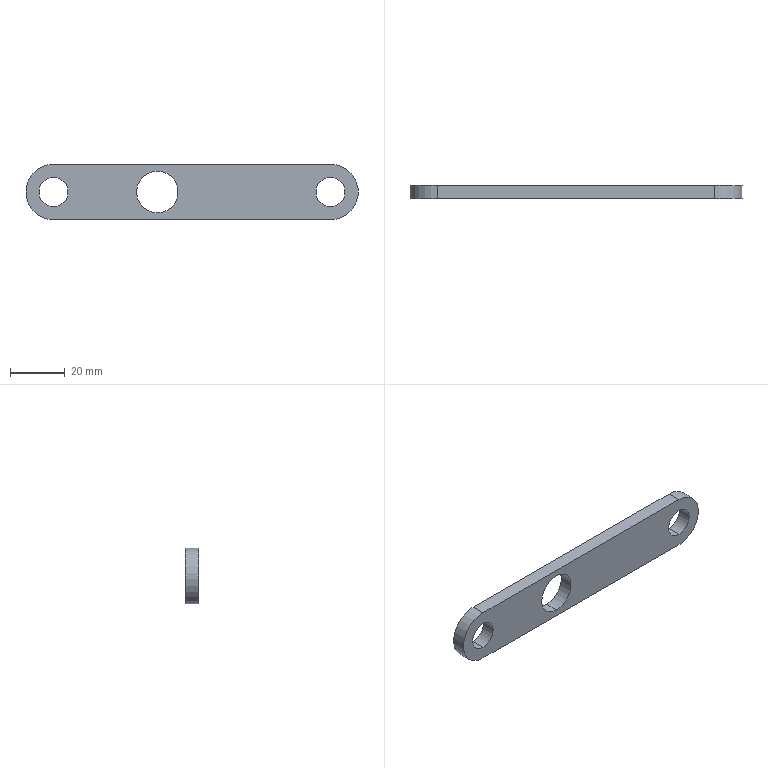Part | SolidWorks | features Extrusion 1, Scale 1 | 1 solid | 12 faces | box 121.92 x 5.08 x 20.32 mm | volume 10300 mm3 | cylinder 8 | plane 4 | commonest cylinder face diameters 10.668 x4 15.24 x2 20.32 x2
STEP:
#1=CARTESIAN_POINT('',(-12.7,5.08,-7.62));
#2=VERTEX_POINT('',#1);
#3=CARTESIAN_POINT('',(-12.7,5.08,7.62));
#4=VERTEX_POINT('',#3);
#5=CARTESIAN_POINT('',(-12.7,5.08,0.));
#6=DIRECTION('',(0.,1.,0.));
#7=DIRECTION('',(0.,0.,1.));
#8=AXIS2_PLACEMENT_3D('',#5,#6,#7);
#9=CIRCLE('',#8,7.62);
#10=EDGE_CURVE('',#2,#4,#9,.T.);
#11=ORIENTED_EDGE('',*,*,#10,.T.);
#12=CARTESIAN_POINT('',(-12.7,0.,7.62));
#13=VERTEX_POINT('',#12);
#14=CARTESIAN_POINT('',(-12.7,5.08,7.62));
#15=DIRECTION('',(0.,-1.,0.));
#16=VECTOR('',#15,1000.);
#17=LINE('',#14,#16);
#18=EDGE_CURVE('',#4,#13,#17,.T.);
#19=ORIENTED_EDGE('',*,*,#18,.T.);
#20=CARTESIAN_POINT('',(-12.7,0.,-7.62));
#21=VERTEX_POINT('',#20);
#22=CARTESIAN_POINT('',(-12.7,0.,0.));
#23=DIRECTION('',(0.,1.,0.));
#24=DIRECTION('',(0.,0.,1.));
#25=AXIS2_PLACEMENT_3D('',#22,#23,#24);
#26=CIRCLE('',#25,7.62);
#27=EDGE_CURVE('',#21,#13,#26,.T.);
#28=ORIENTED_EDGE('',*,*,#27,.F.);
#29=CARTESIAN_POINT('',(-12.7,5.08,-7.62));
#30=DIRECTION('',(0.,-1.,0.));
#31=VECTOR('',#30,1000.);
#32=LINE('',#29,#31);
#33=EDGE_CURVE('',#2,#21,#32,.T.);
#34=ORIENTED_EDGE('',*,*,#33,.F.);
#35=EDGE_LOOP('',(#11,#19,#28,#34));
#36=FACE_OUTER_BOUND('',#35,.T.);
#37=CARTESIAN_POINT('',(-12.7,5.08,0.));
#38=DIRECTION('',(0.,-1.,0.));
#39=DIRECTION('',(0.,0.,-1.));
#40=AXIS2_PLACEMENT_3D('',#37,#38,#39);
#41=CYLINDRICAL_SURFACE('',#40,7.62);
#42=ADVANCED_FACE('',(#36),#41,.F.);
#43=CARTESIAN_POINT('',(50.8,5.08,-5.334));
#44=VERTEX_POINT('',#43);
#45=CARTESIAN_POINT('',(50.8,5.08,5.334));
#46=VERTEX_POINT('',#45);
#47=CARTESIAN_POINT('',(50.8,5.08,0.));
#48=DIRECTION('',(0.,1.,0.));
#49=DIRECTION('',(0.,0.,1.));
#50=AXIS2_PLACEMENT_3D('',#47,#48,#49);
#51=CIRCLE('',#50,5.334);
#52=EDGE_CURVE('',#44,#46,#51,.T.);
#53=ORIENTED_EDGE('',*,*,#52,.T.);
#54=CARTESIAN_POINT('',(50.8,0.,5.334));
#55=VERTEX_POINT('',#54);
#56=CARTESIAN_POINT('',(50.8,5.08,5.334));
#57=DIRECTION('',(0.,-1.,0.));
#58=VECTOR('',#57,1000.);
#59=LINE('',#56,#58);
#60=EDGE_CURVE('',#46,#55,#59,.T.);
#61=ORIENTED_EDGE('',*,*,#60,.T.);
#62=CARTESIAN_POINT('',(50.8,0.,-5.334));
#63=VERTEX_POINT('',#62);
#64=CARTESIAN_POINT('',(50.8,0.,0.));
#65=DIRECTION('',(0.,1.,0.));
#66=DIRECTION('',(0.,0.,1.));
#67=AXIS2_PLACEMENT_3D('',#64,#65,#66);
#68=CIRCLE('',#67,5.334);
#69=EDGE_CURVE('',#63,#55,#68,.T.);
#70=ORIENTED_EDGE('',*,*,#69,.F.);
#71=CARTESIAN_POINT('',(50.8,5.08,-5.334));
#72=DIRECTION('',(0.,-1.,0.));
#73=VECTOR('',#72,1000.);
#74=LINE('',#71,#73);
#75=EDGE_CURVE('',#44,#63,#74,.T.);
#76=ORIENTED_EDGE('',*,*,#75,.F.);
#77=EDGE_LOOP('',(#53,#61,#70,#76));
#78=FACE_OUTER_BOUND('',#77,.T.);
#79=CARTESIAN_POINT('',(50.8,5.08,0.));
#80=DIRECTION('',(0.,-1.,0.));
#81=DIRECTION('',(0.,0.,-1.));
#82=AXIS2_PLACEMENT_3D('',#79,#80,#81);
#83=CYLINDRICAL_SURFACE('',#82,5.334);
#84=ADVANCED_FACE('',(#78),#83,.F.);
#85=CARTESIAN_POINT('',(-50.8,5.08,-5.334));
#86=VERTEX_POINT('',#85);
#87=CARTESIAN_POINT('',(-50.8,5.08,5.334));
#88=VERTEX_POINT('',#87);
#89=CARTESIAN_POINT('',(-50.8,5.08,0.));
#90=DIRECTION('',(0.,1.,0.));
#91=DIRECTION('',(0.,0.,1.));
#92=AXIS2_PLACEMENT_3D('',#89,#90,#91);
#93=CIRCLE('',#92,5.334);
#94=EDGE_CURVE('',#86,#88,#93,.T.);
#95=ORIENTED_EDGE('',*,*,#94,.T.);
#96=CARTESIAN_POINT('',(-50.8,0.,5.334));
#97=VERTEX_POINT('',#96);
#98=CARTESIAN_POINT('',(-50.8,5.08,5.334));
#99=DIRECTION('',(0.,-1.,0.));
#100=VECTOR('',#99,1000.);
#101=LINE('',#98,#100);
#102=EDGE_CURVE('',#88,#97,#101,.T.);
#103=ORIENTED_EDGE('',*,*,#102,.T.);
#104=CARTESIAN_POINT('',(-50.8,0.,-5.334));
#105=VERTEX_POINT('',#104);
#106=CARTESIAN_POINT('',(-50.8,0.,0.));
#107=DIRECTION('',(0.,1.,0.));
#108=DIRECTION('',(0.,0.,1.));
#109=AXIS2_PLACEMENT_3D('',#106,#107,#108);
#110=CIRCLE('',#109,5.334);
#111=EDGE_CURVE('',#105,#97,#110,.T.);
#112=ORIENTED_EDGE('',*,*,#111,.F.);
#113=CARTESIAN_POINT('',(-50.8,5.08,-5.334));
#114=DIRECTION('',(0.,-1.,0.));
#115=VECTOR('',#114,1000.);
#116=LINE('',#113,#115);
#117=EDGE_CURVE('',#86,#105,#116,.T.);
#118=ORIENTED_EDGE('',*,*,#117,.F.);
#119=EDGE_LOOP('',(#95,#103,#112,#118));
#120=FACE_OUTER_BOUND('',#119,.T.);
#121=CARTESIAN_POINT('',(-50.8,5.08,0.));
#122=DIRECTION('',(0.,-1.,0.));
#123=DIRECTION('',(0.,0.,-1.));
#124=AXIS2_PLACEMENT_3D('',#121,#122,#123);
#125=CYLINDRICAL_SURFACE('',#124,5.334);
#126=ADVANCED_FACE('',(#120),#125,.F.);
#127=ORIENTED_EDGE('',*,*,#52,.F.);
#128=CARTESIAN_POINT('',(50.8,5.08,0.));
#129=DIRECTION('',(0.,1.,0.));
#130=DIRECTION('',(0.,0.,1.));
#131=AXIS2_PLACEMENT_3D('',#128,#129,#130);
#132=CIRCLE('',#131,5.334);
#133=EDGE_CURVE('',#46,#44,#132,.T.);
#134=ORIENTED_EDGE('',*,*,#133,.F.);
#135=EDGE_LOOP('',(#127,#134));
#136=FACE_BOUND('',#135,.T.);
#137=CARTESIAN_POINT('',(-50.8,5.08,-10.16));
#138=VERTEX_POINT('',#137);
#139=CARTESIAN_POINT('',(-50.8,5.08,10.16));
#140=VERTEX_POINT('',#139);
#141=CARTESIAN_POINT('',(-50.8,5.08,0.));
#142=DIRECTION('',(0.,1.,0.));
#143=DIRECTION('',(0.,0.,1.));
#144=AXIS2_PLACEMENT_3D('',#141,#142,#143);
#145=CIRCLE('',#144,10.16);
#146=EDGE_CURVE('',#138,#140,#145,.T.);
#147=ORIENTED_EDGE('',*,*,#146,.T.);
#148=CARTESIAN_POINT('',(50.8,5.08,10.16));
#149=VERTEX_POINT('',#148);
#150=CARTESIAN_POINT('',(-50.8,5.08,10.16));
#151=DIRECTION('',(1.,0.,0.));
#152=VECTOR('',#151,1000.);
#153=LINE('',#150,#152);
#154=EDGE_CURVE('',#140,#149,#153,.T.);
#155=ORIENTED_EDGE('',*,*,#154,.T.);
#156=CARTESIAN_POINT('',(50.8,5.08,-10.16));
#157=VERTEX_POINT('',#156);
#158=CARTESIAN_POINT('',(50.8,5.08,0.));
#159=DIRECTION('',(0.,1.,0.));
#160=DIRECTION('',(0.,0.,1.));
#161=AXIS2_PLACEMENT_3D('',#158,#159,#160);
#162=CIRCLE('',#161,10.16);
#163=EDGE_CURVE('',#149,#157,#162,.T.);
#164=ORIENTED_EDGE('',*,*,#163,.T.);
#165=CARTESIAN_POINT('',(-50.8,5.08,-10.16));
#166=DIRECTION('',(-1.,0.,0.));
#167=VECTOR('',#166,1000.);
#168=LINE('',#165,#167);
#169=EDGE_CURVE('',#157,#138,#168,.T.);
#170=ORIENTED_EDGE('',*,*,#169,.T.);
#171=EDGE_LOOP('',(#147,#155,#164,#170));
#172=FACE_OUTER_BOUND('',#171,.T.);
#173=ORIENTED_EDGE('',*,*,#94,.F.);
#174=CARTESIAN_POINT('',(-50.8,5.08,0.));
#175=DIRECTION('',(0.,1.,0.));
#176=DIRECTION('',(0.,0.,1.));
#177=AXIS2_PLACEMENT_3D('',#174,#175,#176);
#178=CIRCLE('',#177,5.334);
#179=EDGE_CURVE('',#88,#86,#178,.T.);
#180=ORIENTED_EDGE('',*,*,#179,.F.);
#181=EDGE_LOOP('',(#173,#180));
#182=FACE_BOUND('',#181,.T.);
#183=ORIENTED_EDGE('',*,*,#10,.F.);
#184=CARTESIAN_POINT('',(-12.7,5.08,0.));
#185=DIRECTION('',(0.,1.,0.));
#186=DIRECTION('',(0.,0.,1.));
#187=AXIS2_PLACEMENT_3D('',#184,#185,#186);
#188=CIRCLE('',#187,7.62);
#189=EDGE_CURVE('',#4,#2,#188,.T.);
#190=ORIENTED_EDGE('',*,*,#189,.F.);
#191=EDGE_LOOP('',(#183,#190));
#192=FACE_BOUND('',#191,.T.);
#193=CARTESIAN_POINT('',(-50.8,5.08,0.));
#194=DIRECTION('',(0.,1.,0.));
#195=DIRECTION('',(0.,0.,1.));
#196=AXIS2_PLACEMENT_3D('',#193,#194,#195);
#197=PLANE('',#196);
#198=ADVANCED_FACE('',(#136,#172,#182,#192),#197,.T.);
#199=ORIENTED_EDGE('',*,*,#69,.T.);
#200=CARTESIAN_POINT('',(50.8,0.,0.));
#201=DIRECTION('',(0.,1.,0.));
#202=DIRECTION('',(0.,0.,1.));
#203=AXIS2_PLACEMENT_3D('',#200,#201,#202);
#204=CIRCLE('',#203,5.334);
#205=EDGE_CURVE('',#55,#63,#204,.T.);
#206=ORIENTED_EDGE('',*,*,#205,.T.);
#207=EDGE_LOOP('',(#199,#206));
#208=FACE_BOUND('',#207,.T.);
#209=CARTESIAN_POINT('',(-50.8,0.,-10.16));
#210=VERTEX_POINT('',#209);
#211=CARTESIAN_POINT('',(-50.8,0.,10.16));
#212=VERTEX_POINT('',#211);
#213=CARTESIAN_POINT('',(-50.8,0.,0.));
#214=DIRECTION('',(0.,1.,0.));
#215=DIRECTION('',(0.,0.,1.));
#216=AXIS2_PLACEMENT_3D('',#213,#214,#215);
#217=CIRCLE('',#216,10.16);
#218=EDGE_CURVE('',#210,#212,#217,.T.);
#219=ORIENTED_EDGE('',*,*,#218,.F.);
#220=CARTESIAN_POINT('',(50.8,0.,-10.16));
#221=VERTEX_POINT('',#220);
#222=CARTESIAN_POINT('',(-50.8,0.,-10.16));
#223=DIRECTION('',(-1.,0.,0.));
#224=VECTOR('',#223,1000.);
#225=LINE('',#222,#224);
#226=EDGE_CURVE('',#221,#210,#225,.T.);
#227=ORIENTED_EDGE('',*,*,#226,.F.);
#228=CARTESIAN_POINT('',(50.8,0.,10.16));
#229=VERTEX_POINT('',#228);
#230=CARTESIAN_POINT('',(50.8,0.,0.));
#231=DIRECTION('',(0.,1.,0.));
#232=DIRECTION('',(0.,0.,1.));
#233=AXIS2_PLACEMENT_3D('',#230,#231,#232);
#234=CIRCLE('',#233,10.16);
#235=EDGE_CURVE('',#229,#221,#234,.T.);
#236=ORIENTED_EDGE('',*,*,#235,.F.);
#237=CARTESIAN_POINT('',(-50.8,0.,10.16));
#238=DIRECTION('',(1.,0.,0.));
#239=VECTOR('',#238,1000.);
#240=LINE('',#237,#239);
#241=EDGE_CURVE('',#212,#229,#240,.T.);
#242=ORIENTED_EDGE('',*,*,#241,.F.);
#243=EDGE_LOOP('',(#219,#227,#236,#242));
#244=FACE_OUTER_BOUND('',#243,.T.);
#245=ORIENTED_EDGE('',*,*,#111,.T.);
#246=CARTESIAN_POINT('',(-50.8,0.,0.));
#247=DIRECTION('',(0.,1.,0.));
#248=DIRECTION('',(0.,0.,1.));
#249=AXIS2_PLACEMENT_3D('',#246,#247,#248);
#250=CIRCLE('',#249,5.334);
#251=EDGE_CURVE('',#97,#105,#250,.T.);
#252=ORIENTED_EDGE('',*,*,#251,.T.);
#253=EDGE_LOOP('',(#245,#252));
#254=FACE_BOUND('',#253,.T.);
#255=ORIENTED_EDGE('',*,*,#27,.T.);
#256=CARTESIAN_POINT('',(-12.7,0.,0.));
#257=DIRECTION('',(0.,1.,0.));
#258=DIRECTION('',(0.,0.,1.));
#259=AXIS2_PLACEMENT_3D('',#256,#257,#258);
#260=CIRCLE('',#259,7.62);
#261=EDGE_CURVE('',#13,#21,#260,.T.);
#262=ORIENTED_EDGE('',*,*,#261,.T.);
#263=EDGE_LOOP('',(#255,#262));
#264=FACE_BOUND('',#263,.T.);
#265=CARTESIAN_POINT('',(-50.8,0.,0.));
#266=DIRECTION('',(0.,1.,0.));
#267=DIRECTION('',(0.,0.,1.));
#268=AXIS2_PLACEMENT_3D('',#265,#266,#267);
#269=PLANE('',#268);
#270=ADVANCED_FACE('',(#208,#244,#254,#264),#269,.F.);
#271=ORIENTED_EDGE('',*,*,#218,.T.);
#272=CARTESIAN_POINT('',(-50.8,5.08,10.16));
#273=DIRECTION('',(0.,-1.,0.));
#274=VECTOR('',#273,1000.);
#275=LINE('',#272,#274);
#276=EDGE_CURVE('',#140,#212,#275,.T.);
#277=ORIENTED_EDGE('',*,*,#276,.F.);
#278=ORIENTED_EDGE('',*,*,#146,.F.);
#279=CARTESIAN_POINT('',(-50.8,5.08,-10.16));
#280=DIRECTION('',(0.,-1.,0.));
#281=VECTOR('',#280,1000.);
#282=LINE('',#279,#281);
#283=EDGE_CURVE('',#138,#210,#282,.T.);
#284=ORIENTED_EDGE('',*,*,#283,.T.);
#285=EDGE_LOOP('',(#271,#277,#278,#284));
#286=FACE_OUTER_BOUND('',#285,.T.);
#287=CARTESIAN_POINT('',(-50.8,5.08,0.));
#288=DIRECTION('',(0.,-1.,0.));
#289=DIRECTION('',(0.,0.,-1.));
#290=AXIS2_PLACEMENT_3D('',#287,#288,#289);
#291=CYLINDRICAL_SURFACE('',#290,10.16);
#292=ADVANCED_FACE('',(#286),#291,.T.);
#293=ORIENTED_EDGE('',*,*,#241,.T.);
#294=CARTESIAN_POINT('',(50.8,5.08,10.16));
#295=DIRECTION('',(0.,-1.,0.));
#296=VECTOR('',#295,1000.);
#297=LINE('',#294,#296);
#298=EDGE_CURVE('',#149,#229,#297,.T.);
#299=ORIENTED_EDGE('',*,*,#298,.F.);
#300=ORIENTED_EDGE('',*,*,#154,.F.);
#301=ORIENTED_EDGE('',*,*,#276,.T.);
#302=EDGE_LOOP('',(#293,#299,#300,#301));
#303=FACE_OUTER_BOUND('',#302,.T.);
#304=CARTESIAN_POINT('',(-50.8,5.08,10.16));
#305=DIRECTION('',(0.,0.,-1.));
#306=DIRECTION('',(-1.,0.,0.));
#307=AXIS2_PLACEMENT_3D('',#304,#305,#306);
#308=PLANE('',#307);
#309=ADVANCED_FACE('',(#303),#308,.F.);
#310=ORIENTED_EDGE('',*,*,#235,.T.);
#311=CARTESIAN_POINT('',(50.8,5.08,-10.16));
#312=DIRECTION('',(0.,-1.,0.));
#313=VECTOR('',#312,1000.);
#314=LINE('',#311,#313);
#315=EDGE_CURVE('',#157,#221,#314,.T.);
#316=ORIENTED_EDGE('',*,*,#315,.F.);
#317=ORIENTED_EDGE('',*,*,#163,.F.);
#318=ORIENTED_EDGE('',*,*,#298,.T.);
#319=EDGE_LOOP('',(#310,#316,#317,#318));
#320=FACE_OUTER_BOUND('',#319,.T.);
#321=CARTESIAN_POINT('',(50.8,5.08,0.));
#322=DIRECTION('',(0.,-1.,0.));
#323=DIRECTION('',(0.,0.,-1.));
#324=AXIS2_PLACEMENT_3D('',#321,#322,#323);
#325=CYLINDRICAL_SURFACE('',#324,10.16);
#326=ADVANCED_FACE('',(#320),#325,.T.);
#327=ORIENTED_EDGE('',*,*,#226,.T.);
#328=ORIENTED_EDGE('',*,*,#283,.F.);
#329=ORIENTED_EDGE('',*,*,#169,.F.);
#330=ORIENTED_EDGE('',*,*,#315,.T.);
#331=EDGE_LOOP('',(#327,#328,#329,#330));
#332=FACE_OUTER_BOUND('',#331,.T.);
#333=CARTESIAN_POINT('',(-50.8,5.08,-10.16));
#334=DIRECTION('',(0.,0.,1.));
#335=DIRECTION('',(1.,0.,0.));
#336=AXIS2_PLACEMENT_3D('',#333,#334,#335);
#337=PLANE('',#336);
#338=ADVANCED_FACE('',(#332),#337,.F.);
#339=ORIENTED_EDGE('',*,*,#102,.F.);
#340=ORIENTED_EDGE('',*,*,#179,.T.);
#341=ORIENTED_EDGE('',*,*,#117,.T.);
#342=ORIENTED_EDGE('',*,*,#251,.F.);
#343=EDGE_LOOP('',(#339,#340,#341,#342));
#344=FACE_OUTER_BOUND('',#343,.T.);
#345=CARTESIAN_POINT('',(-50.8,5.08,0.));
#346=DIRECTION('',(0.,-1.,0.));
#347=DIRECTION('',(0.,0.,-1.));
#348=AXIS2_PLACEMENT_3D('',#345,#346,#347);
#349=CYLINDRICAL_SURFACE('',#348,5.334);
#350=ADVANCED_FACE('',(#344),#349,.F.);
#351=ORIENTED_EDGE('',*,*,#60,.F.);
#352=ORIENTED_EDGE('',*,*,#133,.T.);
#353=ORIENTED_EDGE('',*,*,#75,.T.);
#354=ORIENTED_EDGE('',*,*,#205,.F.);
#355=EDGE_LOOP('',(#351,#352,#353,#354));
#356=FACE_OUTER_BOUND('',#355,.T.);
#357=CARTESIAN_POINT('',(50.8,5.08,0.));
#358=DIRECTION('',(0.,-1.,0.));
#359=DIRECTION('',(0.,0.,-1.));
#360=AXIS2_PLACEMENT_3D('',#357,#358,#359);
#361=CYLINDRICAL_SURFACE('',#360,5.334);
#362=ADVANCED_FACE('',(#356),#361,.F.);
#363=ORIENTED_EDGE('',*,*,#18,.F.);
#364=ORIENTED_EDGE('',*,*,#189,.T.);
#365=ORIENTED_EDGE('',*,*,#33,.T.);
#366=ORIENTED_EDGE('',*,*,#261,.F.);
#367=EDGE_LOOP('',(#363,#364,#365,#366));
#368=FACE_OUTER_BOUND('',#367,.T.);
#369=CARTESIAN_POINT('',(-12.7,5.08,0.));
#370=DIRECTION('',(0.,-1.,0.));
#371=DIRECTION('',(0.,0.,-1.));
#372=AXIS2_PLACEMENT_3D('',#369,#370,#371);
#373=CYLINDRICAL_SURFACE('',#372,7.62);
#374=ADVANCED_FACE('',(#368),#373,.F.);
#375=CLOSED_SHELL('',(#42,#84,#126,#198,#270,#292,#309,#326,#338,#350,#362,#374));
#376=MANIFOLD_SOLID_BREP('',#375);
#377=CARTESIAN_POINT('',(0.,0.,0.));
#378=DIRECTION('',(0.,0.,1.));
#379=DIRECTION('',(1.,0.,0.));
#380=AXIS2_PLACEMENT_3D('',#377,#378,#379);
#381=(LENGTH_UNIT()NAMED_UNIT(*)SI_UNIT(.MILLI.,.METRE.));
#382=UNCERTAINTY_MEASURE_WITH_UNIT(LENGTH_MEASURE(0.00001),#381,'','');
#383=(NAMED_UNIT(*)PLANE_ANGLE_UNIT()SI_UNIT($,.RADIAN.));
#384=(NAMED_UNIT(*)SI_UNIT($,.STERADIAN.)SOLID_ANGLE_UNIT());
#385=(GEOMETRIC_REPRESENTATION_CONTEXT(3)GLOBAL_UNCERTAINTY_ASSIGNED_CONTEXT((#382))GLOBAL_UNIT_ASSIGNED_CONTEXT((#381,#383,#384))REPRESENTATION_CONTEXT('',''));
#386=ADVANCED_BREP_SHAPE_REPRESENTATION('',(#376,#380),#385);